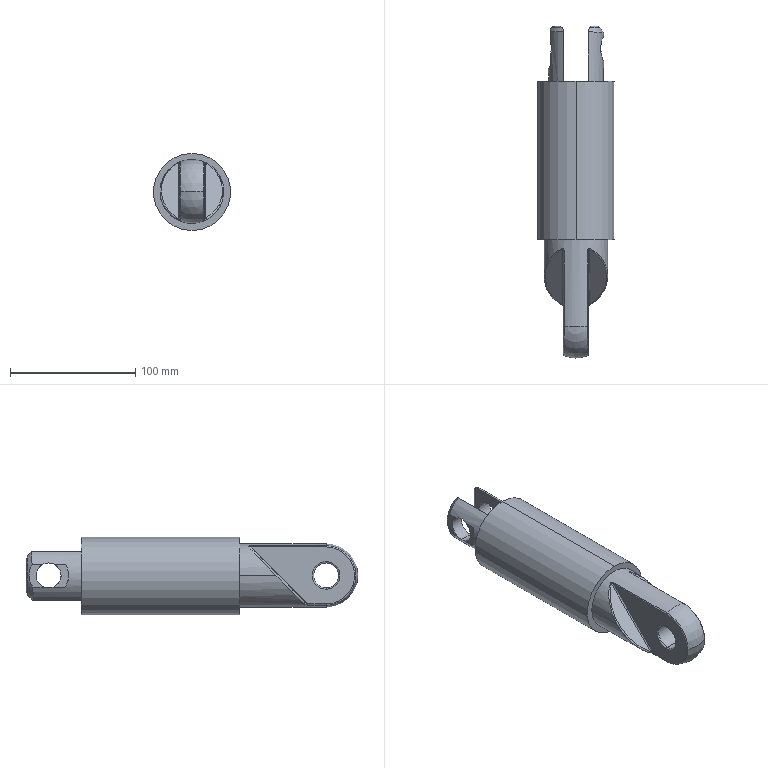Part | SolidWorks | features ICE 11, Fillet 2, MirrorPattern 1, MoveCopyBody 1, Revolution 1, Scale 1, Split 1 | 1 solid | 60 faces | box 61.465 x 264.6 x 61.465 mm | volume 508249 mm3 | cylinder 25 | plane 14 | torus 9 | sphere 6 | spline 6 | commonest cylinder face diameters 2 x6 20 x6 50.8 x4 8 x2 43.949 x2 50 x2